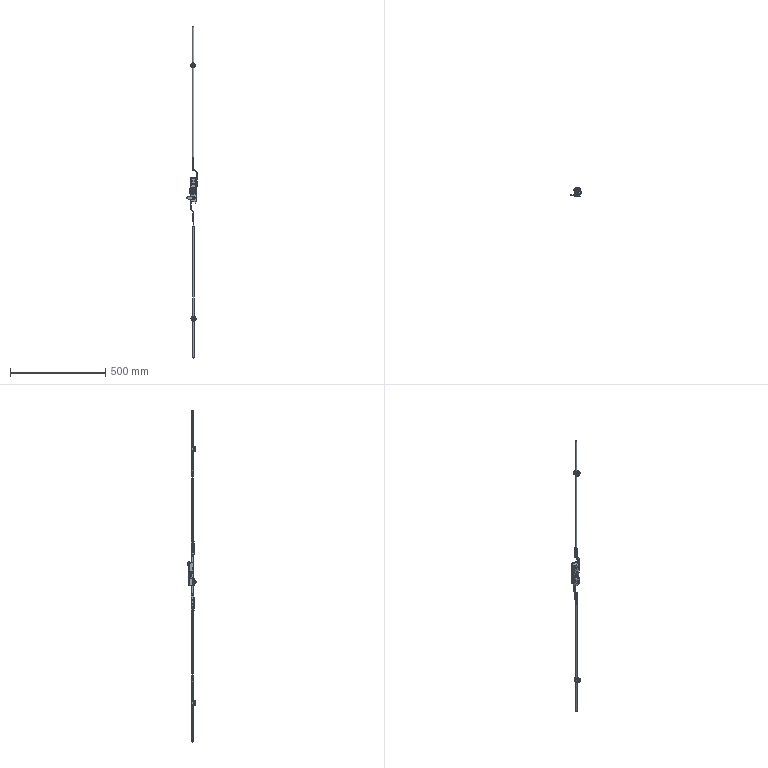Part | SolidWorks | 5 solids | 1030 faces | box 55.3 x 46.477 x 1742 mm | volume 177149 mm3 | cylinder 427 | plane 396 | spline 178 | cone 29 | commonest cylinder face diameters 1 x144 0.8 x52 6.1 x46 2 x26 16 x26 1.6 x24